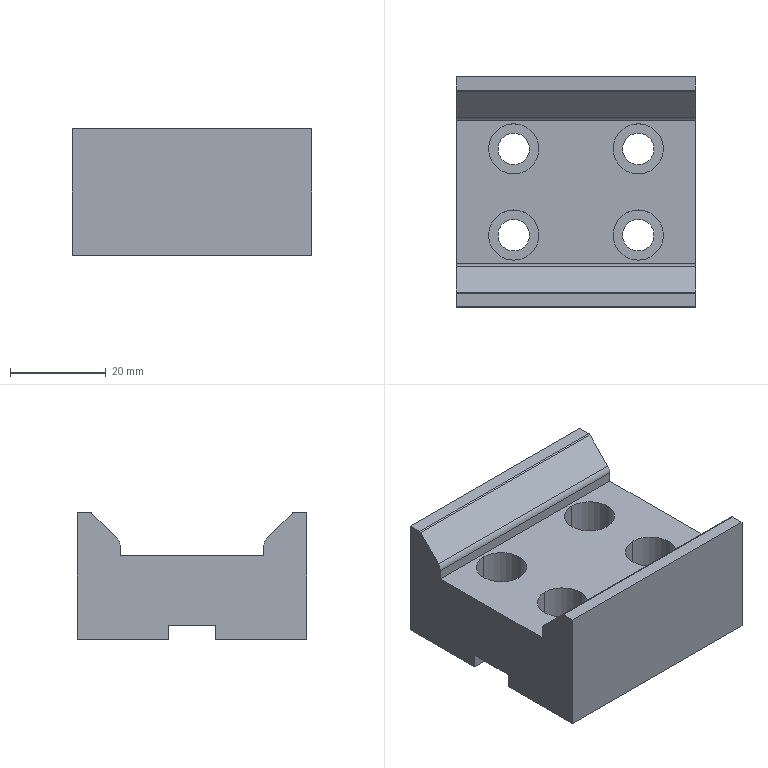Part | STEP file | J454-EBZ05-20-03-Part-1-4 | 1 solid | 40 faces | box 50 x 48 x 26.5 mm | volume 42271 mm3 | cylinder 20 | plane 20 | commonest cylinder face diameters 6.6 x8 10.5 x8 1 x2 4 x2